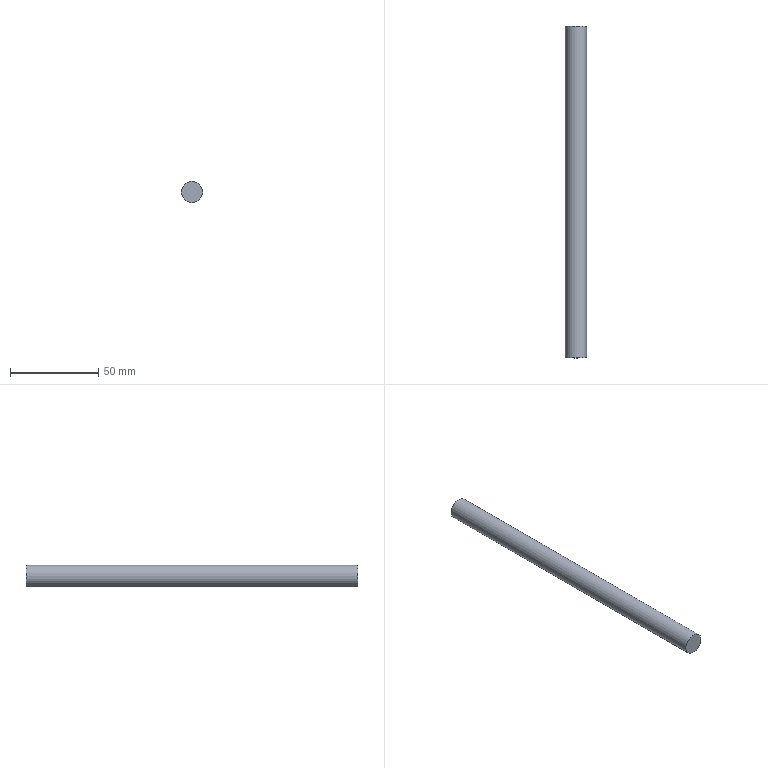Part | STEP file | 冲床-300配套压波_id282_x_t | 1 solid | 3 faces | box 12 x 188 x 12 mm | volume 21262 mm3 | plane 2 | cylinder 1 | commonest cylinder face diameters 12 x1
STEP:
#1=CARTESIAN_POINT('',(1151.,70.,229.));
#2=VERTEX_POINT('',#1);
#3=CARTESIAN_POINT('',(1157.,70.,229.));
#4=DIRECTION('',(0.,1.,0.));
#5=DIRECTION('',(-1.,0.,0.));
#6=AXIS2_PLACEMENT_3D('',#3,#4,#5);
#7=CIRCLE('',#6,6.);
#8=EDGE_CURVE('',#2,#2,#7,.T.);
#9=ORIENTED_EDGE('',*,*,#8,.F.);
#10=EDGE_LOOP('',(#9));
#11=FACE_BOUND('',#10,.T.);
#12=CARTESIAN_POINT('',(1151.,-118.,229.));
#13=VERTEX_POINT('',#12);
#14=CARTESIAN_POINT('',(1157.,-118.,229.));
#15=DIRECTION('',(0.,1.,0.));
#16=DIRECTION('',(-1.,0.,0.));
#17=AXIS2_PLACEMENT_3D('',#14,#15,#16);
#18=CIRCLE('',#17,6.);
#19=EDGE_CURVE('',#13,#13,#18,.T.);
#20=ORIENTED_EDGE('',*,*,#19,.T.);
#21=EDGE_LOOP('',(#20));
#22=FACE_BOUND('',#21,.T.);
#23=CARTESIAN_POINT('',(1157.,70.,229.));
#24=DIRECTION('',(0.,-1.,0.));
#25=DIRECTION('',(0.,0.,-1.));
#26=AXIS2_PLACEMENT_3D('',#23,#24,#25);
#27=CYLINDRICAL_SURFACE('',#26,6.);
#28=ADVANCED_FACE('',(#11,#22),#27,.T.);
#29=ORIENTED_EDGE('',*,*,#8,.T.);
#30=EDGE_LOOP('',(#29));
#31=FACE_OUTER_BOUND('',#30,.T.);
#32=CARTESIAN_POINT('',(1157.,70.,229.));
#33=DIRECTION('',(0.,1.,0.));
#34=DIRECTION('',(0.,0.,1.));
#35=AXIS2_PLACEMENT_3D('',#32,#33,#34);
#36=PLANE('',#35);
#37=ADVANCED_FACE('',(#31),#36,.T.);
#38=ORIENTED_EDGE('',*,*,#19,.F.);
#39=EDGE_LOOP('',(#38));
#40=FACE_OUTER_BOUND('',#39,.T.);
#41=CARTESIAN_POINT('',(1157.,-118.,229.));
#42=DIRECTION('',(0.,1.,0.));
#43=DIRECTION('',(0.,0.,1.));
#44=AXIS2_PLACEMENT_3D('',#41,#42,#43);
#45=PLANE('',#44);
#46=ADVANCED_FACE('',(#40),#45,.F.);
#47=CLOSED_SHELL('',(#28,#37,#46));
#48=MANIFOLD_SOLID_BREP('',#47);
#49=(LENGTH_UNIT()NAMED_UNIT(*)SI_UNIT(.MILLI.,.METRE.));
#50=UNCERTAINTY_MEASURE_WITH_UNIT(LENGTH_MEASURE(0.00002),#49,'','');
#51=(NAMED_UNIT(*)PLANE_ANGLE_UNIT()SI_UNIT($,.RADIAN.));
#52=PLANE_ANGLE_MEASURE_WITH_UNIT(PLANE_ANGLE_MEASURE(0.01745),#51);
#53=DIMENSIONAL_EXPONENTS(0.,0.,0.,0.,0.,0.,0.);
#54=(CONVERSION_BASED_UNIT('DEGREE',#52)NAMED_UNIT(#53)PLANE_ANGLE_UNIT());
#55=(NAMED_UNIT(*)SI_UNIT($,.STERADIAN.)SOLID_ANGLE_UNIT());
#56=(GEOMETRIC_REPRESENTATION_CONTEXT(3)GLOBAL_UNCERTAINTY_ASSIGNED_CONTEXT((#50))GLOBAL_UNIT_ASSIGNED_CONTEXT((#49,#54,#55))REPRESENTATION_CONTEXT('',''));
#57=ADVANCED_BREP_SHAPE_REPRESENTATION('',(#48),#56);